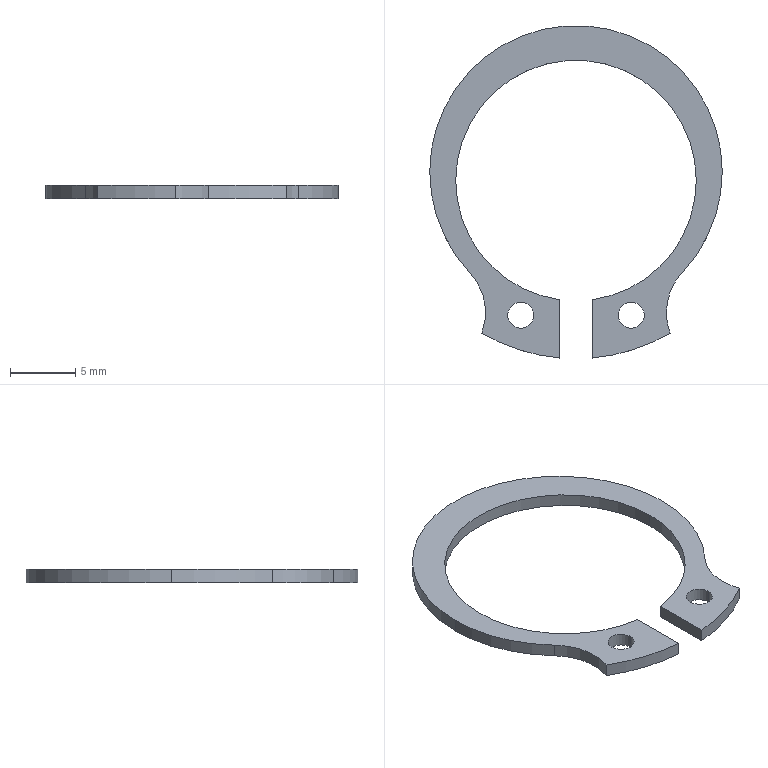Part | STEP file | 1 solid | 19 faces | box 22.5 x 25.566 x 1 mm | volume 158.597 mm3 | cylinder 15 | plane 4 | commonest cylinder face diameters 2 x4 9 x3 18.5 x3 22.5 x3 28.74 x2
STEP:
#1=CARTESIAN_POINT('',(3.25,-11.032,0.5));
#2=VERTEX_POINT('',#1);
#3=CARTESIAN_POINT('',(5.25,-11.032,0.5));
#4=VERTEX_POINT('',#3);
#5=CARTESIAN_POINT('',(4.25,-11.032,0.5));
#6=DIRECTION('',(0.,0.,1.));
#7=DIRECTION('',(-1.,0.,0.));
#8=AXIS2_PLACEMENT_3D('',#5,#6,#7);
#9=CIRCLE('',#8,1.);
#10=EDGE_CURVE('',#2,#4,#9,.T.);
#11=ORIENTED_EDGE('',*,*,#10,.T.);
#12=CARTESIAN_POINT('',(5.25,-11.032,-0.5));
#13=VERTEX_POINT('',#12);
#14=CARTESIAN_POINT('',(5.25,-11.032,0.5));
#15=DIRECTION('',(0.,0.,-1.));
#16=VECTOR('',#15,1000.);
#17=LINE('',#14,#16);
#18=EDGE_CURVE('',#4,#13,#17,.T.);
#19=ORIENTED_EDGE('',*,*,#18,.T.);
#20=CARTESIAN_POINT('',(3.25,-11.032,-0.5));
#21=VERTEX_POINT('',#20);
#22=CARTESIAN_POINT('',(4.25,-11.032,-0.5));
#23=DIRECTION('',(0.,0.,1.));
#24=DIRECTION('',(-1.,0.,0.));
#25=AXIS2_PLACEMENT_3D('',#22,#23,#24);
#26=CIRCLE('',#25,1.);
#27=EDGE_CURVE('',#21,#13,#26,.T.);
#28=ORIENTED_EDGE('',*,*,#27,.F.);
#29=CARTESIAN_POINT('',(3.25,-11.032,0.5));
#30=DIRECTION('',(0.,0.,-1.));
#31=VECTOR('',#30,1000.);
#32=LINE('',#29,#31);
#33=EDGE_CURVE('',#2,#21,#32,.T.);
#34=ORIENTED_EDGE('',*,*,#33,.F.);
#35=EDGE_LOOP('',(#11,#19,#28,#34));
#36=FACE_OUTER_BOUND('',#35,.T.);
#37=CARTESIAN_POINT('',(4.25,-11.032,0.5));
#38=DIRECTION('',(0.,0.,-1.));
#39=DIRECTION('',(-1.,0.,0.));
#40=AXIS2_PLACEMENT_3D('',#37,#38,#39);
#41=CYLINDRICAL_SURFACE('',#40,1.);
#42=ADVANCED_FACE('',(#36),#41,.F.);
#43=CARTESIAN_POINT('',(-5.25,-11.032,0.5));
#44=VERTEX_POINT('',#43);
#45=CARTESIAN_POINT('',(-3.25,-11.032,0.5));
#46=VERTEX_POINT('',#45);
#47=CARTESIAN_POINT('',(-4.25,-11.032,0.5));
#48=DIRECTION('',(0.,0.,1.));
#49=DIRECTION('',(1.,0.,0.));
#50=AXIS2_PLACEMENT_3D('',#47,#48,#49);
#51=CIRCLE('',#50,1.);
#52=EDGE_CURVE('',#44,#46,#51,.T.);
#53=ORIENTED_EDGE('',*,*,#52,.T.);
#54=CARTESIAN_POINT('',(-3.25,-11.032,-0.5));
#55=VERTEX_POINT('',#54);
#56=CARTESIAN_POINT('',(-3.25,-11.032,0.5));
#57=DIRECTION('',(0.,0.,-1.));
#58=VECTOR('',#57,1000.);
#59=LINE('',#56,#58);
#60=EDGE_CURVE('',#46,#55,#59,.T.);
#61=ORIENTED_EDGE('',*,*,#60,.T.);
#62=CARTESIAN_POINT('',(-5.25,-11.032,-0.5));
#63=VERTEX_POINT('',#62);
#64=CARTESIAN_POINT('',(-4.25,-11.032,-0.5));
#65=DIRECTION('',(0.,0.,1.));
#66=DIRECTION('',(1.,0.,0.));
#67=AXIS2_PLACEMENT_3D('',#64,#65,#66);
#68=CIRCLE('',#67,1.);
#69=EDGE_CURVE('',#63,#55,#68,.T.);
#70=ORIENTED_EDGE('',*,*,#69,.F.);
#71=CARTESIAN_POINT('',(-5.25,-11.032,0.5));
#72=DIRECTION('',(0.,0.,-1.));
#73=VECTOR('',#72,1000.);
#74=LINE('',#71,#73);
#75=EDGE_CURVE('',#44,#63,#74,.T.);
#76=ORIENTED_EDGE('',*,*,#75,.F.);
#77=EDGE_LOOP('',(#53,#61,#70,#76));
#78=FACE_OUTER_BOUND('',#77,.T.);
#79=CARTESIAN_POINT('',(-4.25,-11.032,0.5));
#80=DIRECTION('',(0.,0.,-1.));
#81=DIRECTION('',(-1.,0.,0.));
#82=AXIS2_PLACEMENT_3D('',#79,#80,#81);
#83=CYLINDRICAL_SURFACE('',#82,1.);
#84=ADVANCED_FACE('',(#78),#83,.F.);
#85=CARTESIAN_POINT('',(11.25,0.,0.5));
#86=VERTEX_POINT('',#85);
#87=CARTESIAN_POINT('',(-11.25,0.,0.5));
#88=VERTEX_POINT('',#87);
#89=CARTESIAN_POINT('',(0.,0.,0.5));
#90=DIRECTION('',(0.,0.,1.));
#91=DIRECTION('',(1.,0.,0.));
#92=AXIS2_PLACEMENT_3D('',#89,#90,#91);
#93=CIRCLE('',#92,11.25);
#94=EDGE_CURVE('',#86,#88,#93,.T.);
#95=ORIENTED_EDGE('',*,*,#94,.F.);
#96=CARTESIAN_POINT('',(11.25,0.,-0.5));
#97=VERTEX_POINT('',#96);
#98=CARTESIAN_POINT('',(11.25,0.,0.5));
#99=DIRECTION('',(0.,0.,-1.));
#100=VECTOR('',#99,1000.);
#101=LINE('',#98,#100);
#102=EDGE_CURVE('',#86,#97,#101,.T.);
#103=ORIENTED_EDGE('',*,*,#102,.T.);
#104=CARTESIAN_POINT('',(-11.25,0.,-0.5));
#105=VERTEX_POINT('',#104);
#106=CARTESIAN_POINT('',(0.,0.,-0.5));
#107=DIRECTION('',(0.,0.,1.));
#108=DIRECTION('',(1.,0.,0.));
#109=AXIS2_PLACEMENT_3D('',#106,#107,#108);
#110=CIRCLE('',#109,11.25);
#111=EDGE_CURVE('',#97,#105,#110,.T.);
#112=ORIENTED_EDGE('',*,*,#111,.T.);
#113=CARTESIAN_POINT('',(-11.25,0.,0.5));
#114=DIRECTION('',(0.,0.,-1.));
#115=VECTOR('',#114,1000.);
#116=LINE('',#113,#115);
#117=EDGE_CURVE('',#88,#105,#116,.T.);
#118=ORIENTED_EDGE('',*,*,#117,.F.);
#119=EDGE_LOOP('',(#95,#103,#112,#118));
#120=FACE_OUTER_BOUND('',#119,.T.);
#121=CARTESIAN_POINT('',(0.,0.,0.5));
#122=DIRECTION('',(0.,0.,-1.));
#123=DIRECTION('',(-1.,0.,0.));
#124=AXIS2_PLACEMENT_3D('',#121,#122,#123);
#125=CYLINDRICAL_SURFACE('',#124,11.25);
#126=ADVANCED_FACE('',(#120),#125,.T.);
#127=CARTESIAN_POINT('',(-8.183,-7.72,0.5));
#128=VERTEX_POINT('',#127);
#129=CARTESIAN_POINT('',(0.,0.,0.5));
#130=DIRECTION('',(0.,0.,1.));
#131=DIRECTION('',(1.,0.,0.));
#132=AXIS2_PLACEMENT_3D('',#129,#130,#131);
#133=CIRCLE('',#132,11.25);
#134=EDGE_CURVE('',#88,#128,#133,.T.);
#135=ORIENTED_EDGE('',*,*,#134,.F.);
#136=ORIENTED_EDGE('',*,*,#117,.T.);
#137=CARTESIAN_POINT('',(-8.183,-7.72,-0.5));
#138=VERTEX_POINT('',#137);
#139=CARTESIAN_POINT('',(0.,0.,-0.5));
#140=DIRECTION('',(0.,0.,1.));
#141=DIRECTION('',(1.,0.,0.));
#142=AXIS2_PLACEMENT_3D('',#139,#140,#141);
#143=CIRCLE('',#142,11.25);
#144=EDGE_CURVE('',#105,#138,#143,.T.);
#145=ORIENTED_EDGE('',*,*,#144,.T.);
#146=CARTESIAN_POINT('',(-8.183,-7.72,0.5));
#147=DIRECTION('',(0.,0.,-1.));
#148=VECTOR('',#147,1000.);
#149=LINE('',#146,#148);
#150=EDGE_CURVE('',#128,#138,#149,.T.);
#151=ORIENTED_EDGE('',*,*,#150,.F.);
#152=EDGE_LOOP('',(#135,#136,#145,#151));
#153=FACE_OUTER_BOUND('',#152,.T.);
#154=CARTESIAN_POINT('',(0.,0.,0.5));
#155=DIRECTION('',(0.,0.,-1.));
#156=DIRECTION('',(-1.,0.,0.));
#157=AXIS2_PLACEMENT_3D('',#154,#155,#156);
#158=CYLINDRICAL_SURFACE('',#157,11.25);
#159=ADVANCED_FACE('',(#153),#158,.T.);
#160=CARTESIAN_POINT('',(6.956,-10.808,0.5));
#161=VERTEX_POINT('',#160);
#162=CARTESIAN_POINT('',(8.183,-7.72,0.5));
#163=VERTEX_POINT('',#162);
#164=CARTESIAN_POINT('',(11.456,-10.808,0.5));
#165=DIRECTION('',(0.,0.,-1.));
#166=DIRECTION('',(-1.,0.,0.));
#167=AXIS2_PLACEMENT_3D('',#164,#165,#166);
#168=CIRCLE('',#167,4.5);
#169=EDGE_CURVE('',#161,#163,#168,.T.);
#170=ORIENTED_EDGE('',*,*,#169,.F.);
#171=CARTESIAN_POINT('',(6.956,-10.808,-0.5));
#172=VERTEX_POINT('',#171);
#173=CARTESIAN_POINT('',(6.956,-10.808,0.5));
#174=DIRECTION('',(0.,0.,-1.));
#175=VECTOR('',#174,1000.);
#176=LINE('',#173,#175);
#177=EDGE_CURVE('',#161,#172,#176,.T.);
#178=ORIENTED_EDGE('',*,*,#177,.T.);
#179=CARTESIAN_POINT('',(8.183,-7.72,-0.5));
#180=VERTEX_POINT('',#179);
#181=CARTESIAN_POINT('',(11.456,-10.808,-0.5));
#182=DIRECTION('',(0.,0.,-1.));
#183=DIRECTION('',(-1.,0.,0.));
#184=AXIS2_PLACEMENT_3D('',#181,#182,#183);
#185=CIRCLE('',#184,4.5);
#186=EDGE_CURVE('',#172,#180,#185,.T.);
#187=ORIENTED_EDGE('',*,*,#186,.T.);
#188=CARTESIAN_POINT('',(8.183,-7.72,0.5));
#189=DIRECTION('',(0.,0.,-1.));
#190=VECTOR('',#189,1000.);
#191=LINE('',#188,#190);
#192=EDGE_CURVE('',#163,#180,#191,.T.);
#193=ORIENTED_EDGE('',*,*,#192,.F.);
#194=EDGE_LOOP('',(#170,#178,#187,#193));
#195=FACE_OUTER_BOUND('',#194,.T.);
#196=CARTESIAN_POINT('',(11.456,-10.808,0.5));
#197=DIRECTION('',(0.,0.,-1.));
#198=DIRECTION('',(-1.,0.,0.));
#199=AXIS2_PLACEMENT_3D('',#196,#197,#198);
#200=CYLINDRICAL_SURFACE('',#199,4.5);
#201=ADVANCED_FACE('',(#195),#200,.F.);
#202=CARTESIAN_POINT('',(9.25,-0.67,0.5));
#203=VERTEX_POINT('',#202);
#204=CARTESIAN_POINT('',(1.25,-9.835,0.5));
#205=VERTEX_POINT('',#204);
#206=CARTESIAN_POINT('',(0.,-0.67,0.5));
#207=DIRECTION('',(0.,0.,-1.));
#208=DIRECTION('',(1.,0.,0.));
#209=AXIS2_PLACEMENT_3D('',#206,#207,#208);
#210=CIRCLE('',#209,9.25);
#211=EDGE_CURVE('',#203,#205,#210,.T.);
#212=ORIENTED_EDGE('',*,*,#211,.F.);
#213=CARTESIAN_POINT('',(9.25,-0.67,-0.5));
#214=VERTEX_POINT('',#213);
#215=CARTESIAN_POINT('',(9.25,-0.67,0.5));
#216=DIRECTION('',(0.,0.,-1.));
#217=VECTOR('',#216,1000.);
#218=LINE('',#215,#217);
#219=EDGE_CURVE('',#203,#214,#218,.T.);
#220=ORIENTED_EDGE('',*,*,#219,.T.);
#221=CARTESIAN_POINT('',(1.25,-9.835,-0.5));
#222=VERTEX_POINT('',#221);
#223=CARTESIAN_POINT('',(0.,-0.67,-0.5));
#224=DIRECTION('',(0.,0.,-1.));
#225=DIRECTION('',(1.,0.,0.));
#226=AXIS2_PLACEMENT_3D('',#223,#224,#225);
#227=CIRCLE('',#226,9.25);
#228=EDGE_CURVE('',#214,#222,#227,.T.);
#229=ORIENTED_EDGE('',*,*,#228,.T.);
#230=CARTESIAN_POINT('',(1.25,-9.835,0.5));
#231=DIRECTION('',(0.,0.,-1.));
#232=VECTOR('',#231,1000.);
#233=LINE('',#230,#232);
#234=EDGE_CURVE('',#205,#222,#233,.T.);
#235=ORIENTED_EDGE('',*,*,#234,.F.);
#236=EDGE_LOOP('',(#212,#220,#229,#235));
#237=FACE_OUTER_BOUND('',#236,.T.);
#238=CARTESIAN_POINT('',(0.,-0.67,0.5));
#239=DIRECTION('',(0.,0.,-1.));
#240=DIRECTION('',(-1.,0.,0.));
#241=AXIS2_PLACEMENT_3D('',#238,#239,#240);
#242=CYLINDRICAL_SURFACE('',#241,9.25);
#243=ADVANCED_FACE('',(#237),#242,.F.);
#244=ORIENTED_EDGE('',*,*,#219,.F.);
#245=CARTESIAN_POINT('',(-9.25,-0.67,0.5));
#246=VERTEX_POINT('',#245);
#247=CARTESIAN_POINT('',(0.,-0.67,0.5));
#248=DIRECTION('',(0.,0.,-1.));
#249=DIRECTION('',(1.,0.,0.));
#250=AXIS2_PLACEMENT_3D('',#247,#248,#249);
#251=CIRCLE('',#250,9.25);
#252=EDGE_CURVE('',#246,#203,#251,.T.);
#253=ORIENTED_EDGE('',*,*,#252,.F.);
#254=CARTESIAN_POINT('',(-9.25,-0.67,-0.5));
#255=VERTEX_POINT('',#254);
#256=CARTESIAN_POINT('',(-9.25,-0.67,0.5));
#257=DIRECTION('',(0.,0.,-1.));
#258=VECTOR('',#257,1000.);
#259=LINE('',#256,#258);
#260=EDGE_CURVE('',#246,#255,#259,.T.);
#261=ORIENTED_EDGE('',*,*,#260,.T.);
#262=CARTESIAN_POINT('',(0.,-0.67,-0.5));
#263=DIRECTION('',(0.,0.,-1.));
#264=DIRECTION('',(1.,0.,0.));
#265=AXIS2_PLACEMENT_3D('',#262,#263,#264);
#266=CIRCLE('',#265,9.25);
#267=EDGE_CURVE('',#255,#214,#266,.T.);
#268=ORIENTED_EDGE('',*,*,#267,.T.);
#269=EDGE_LOOP('',(#244,#253,#261,#268));
#270=FACE_OUTER_BOUND('',#269,.T.);
#271=CARTESIAN_POINT('',(0.,-0.67,0.5));
#272=DIRECTION('',(0.,0.,-1.));
#273=DIRECTION('',(-1.,0.,0.));
#274=AXIS2_PLACEMENT_3D('',#271,#272,#273);
#275=CYLINDRICAL_SURFACE('',#274,9.25);
#276=ADVANCED_FACE('',(#270),#275,.F.);
#277=ORIENTED_EDGE('',*,*,#52,.F.);
#278=CARTESIAN_POINT('',(-4.25,-11.032,0.5));
#279=DIRECTION('',(0.,0.,1.));
#280=DIRECTION('',(1.,0.,0.));
#281=AXIS2_PLACEMENT_3D('',#278,#279,#280);
#282=CIRCLE('',#281,1.);
#283=EDGE_CURVE('',#46,#44,#282,.T.);
#284=ORIENTED_EDGE('',*,*,#283,.F.);
#285=EDGE_LOOP('',(#277,#284));
#286=FACE_BOUND('',#285,.T.);
#287=CARTESIAN_POINT('',(-1.25,-9.835,0.5));
#288=VERTEX_POINT('',#287);
#289=CARTESIAN_POINT('',(0.,-0.67,0.5));
#290=DIRECTION('',(0.,0.,-1.));
#291=DIRECTION('',(1.,0.,0.));
#292=AXIS2_PLACEMENT_3D('',#289,#290,#291);
#293=CIRCLE('',#292,9.25);
#294=EDGE_CURVE('',#288,#246,#293,.T.);
#295=ORIENTED_EDGE('',*,*,#294,.T.);
#296=ORIENTED_EDGE('',*,*,#252,.T.);
#297=ORIENTED_EDGE('',*,*,#211,.T.);
#298=CARTESIAN_POINT('',(1.25,-14.316,0.5));
#299=VERTEX_POINT('',#298);
#300=CARTESIAN_POINT('',(1.25,-9.835,0.5));
#301=DIRECTION('',(0.,-1.,0.));
#302=VECTOR('',#301,1000.);
#303=LINE('',#300,#302);
#304=EDGE_CURVE('',#205,#299,#303,.T.);
#305=ORIENTED_EDGE('',*,*,#304,.T.);
#306=CARTESIAN_POINT('',(7.25,-12.407,0.5));
#307=VERTEX_POINT('',#306);
#308=CARTESIAN_POINT('',(0.,0.,0.5));
#309=DIRECTION('',(0.,0.,1.));
#310=DIRECTION('',(1.,0.,0.));
#311=AXIS2_PLACEMENT_3D('',#308,#309,#310);
#312=CIRCLE('',#311,14.37);
#313=EDGE_CURVE('',#299,#307,#312,.T.);
#314=ORIENTED_EDGE('',*,*,#313,.T.);
#315=CARTESIAN_POINT('',(11.456,-10.808,0.5));
#316=DIRECTION('',(0.,0.,-1.));
#317=DIRECTION('',(-1.,0.,0.));
#318=AXIS2_PLACEMENT_3D('',#315,#316,#317);
#319=CIRCLE('',#318,4.5);
#320=EDGE_CURVE('',#307,#161,#319,.T.);
#321=ORIENTED_EDGE('',*,*,#320,.T.);
#322=ORIENTED_EDGE('',*,*,#169,.T.);
#323=CARTESIAN_POINT('',(0.,0.,0.5));
#324=DIRECTION('',(0.,0.,1.));
#325=DIRECTION('',(1.,0.,0.));
#326=AXIS2_PLACEMENT_3D('',#323,#324,#325);
#327=CIRCLE('',#326,11.25);
#328=EDGE_CURVE('',#163,#86,#327,.T.);
#329=ORIENTED_EDGE('',*,*,#328,.T.);
#330=ORIENTED_EDGE('',*,*,#94,.T.);
#331=ORIENTED_EDGE('',*,*,#134,.T.);
#332=CARTESIAN_POINT('',(-7.25,-12.407,0.5));
#333=VERTEX_POINT('',#332);
#334=CARTESIAN_POINT('',(-11.456,-10.808,0.5));
#335=DIRECTION('',(0.,0.,-1.));
#336=DIRECTION('',(1.,0.,0.));
#337=AXIS2_PLACEMENT_3D('',#334,#335,#336);
#338=CIRCLE('',#337,4.5);
#339=EDGE_CURVE('',#128,#333,#338,.T.);
#340=ORIENTED_EDGE('',*,*,#339,.T.);
#341=CARTESIAN_POINT('',(-1.25,-14.316,0.5));
#342=VERTEX_POINT('',#341);
#343=CARTESIAN_POINT('',(0.,0.,0.5));
#344=DIRECTION('',(0.,0.,1.));
#345=DIRECTION('',(-1.,0.,0.));
#346=AXIS2_PLACEMENT_3D('',#343,#344,#345);
#347=CIRCLE('',#346,14.37);
#348=EDGE_CURVE('',#333,#342,#347,.T.);
#349=ORIENTED_EDGE('',*,*,#348,.T.);
#350=CARTESIAN_POINT('',(-1.25,-9.835,0.5));
#351=DIRECTION('',(0.,1.,0.));
#352=VECTOR('',#351,1000.);
#353=LINE('',#350,#352);
#354=EDGE_CURVE('',#342,#288,#353,.T.);
#355=ORIENTED_EDGE('',*,*,#354,.T.);
#356=EDGE_LOOP('',(#295,#296,#297,#305,#314,#321,#322,#329,#330,#331,#340,#349,#355));
#357=FACE_OUTER_BOUND('',#356,.T.);
#358=ORIENTED_EDGE('',*,*,#10,.F.);
#359=CARTESIAN_POINT('',(4.25,-11.032,0.5));
#360=DIRECTION('',(0.,0.,1.));
#361=DIRECTION('',(-1.,0.,0.));
#362=AXIS2_PLACEMENT_3D('',#359,#360,#361);
#363=CIRCLE('',#362,1.);
#364=EDGE_CURVE('',#4,#2,#363,.T.);
#365=ORIENTED_EDGE('',*,*,#364,.F.);
#366=EDGE_LOOP('',(#358,#365));
#367=FACE_BOUND('',#366,.T.);
#368=CARTESIAN_POINT('',(0.,-0.67,0.5));
#369=DIRECTION('',(0.,0.,1.));
#370=DIRECTION('',(1.,0.,0.));
#371=AXIS2_PLACEMENT_3D('',#368,#369,#370);
#372=PLANE('',#371);
#373=ADVANCED_FACE('',(#286,#357,#367),#372,.T.);
#374=ORIENTED_EDGE('',*,*,#260,.F.);
#375=ORIENTED_EDGE('',*,*,#294,.F.);
#376=CARTESIAN_POINT('',(-1.25,-9.835,-0.5));
#377=VERTEX_POINT('',#376);
#378=CARTESIAN_POINT('',(-1.25,-9.835,0.5));
#379=DIRECTION('',(0.,0.,-1.));
#380=VECTOR('',#379,1000.);
#381=LINE('',#378,#380);
#382=EDGE_CURVE('',#288,#377,#381,.T.);
#383=ORIENTED_EDGE('',*,*,#382,.T.);
#384=CARTESIAN_POINT('',(0.,-0.67,-0.5));
#385=DIRECTION('',(0.,0.,-1.));
#386=DIRECTION('',(1.,0.,0.));
#387=AXIS2_PLACEMENT_3D('',#384,#385,#386);
#388=CIRCLE('',#387,9.25);
#389=EDGE_CURVE('',#377,#255,#388,.T.);
#390=ORIENTED_EDGE('',*,*,#389,.T.);
#391=EDGE_LOOP('',(#374,#375,#383,#390));
#392=FACE_OUTER_BOUND('',#391,.T.);
#393=CARTESIAN_POINT('',(0.,-0.67,0.5));
#394=DIRECTION('',(0.,0.,-1.));
#395=DIRECTION('',(-1.,0.,0.));
#396=AXIS2_PLACEMENT_3D('',#393,#394,#395);
#397=CYLINDRICAL_SURFACE('',#396,9.25);
#398=ADVANCED_FACE('',(#392),#397,.F.);
#399=ORIENTED_EDGE('',*,*,#234,.T.);
#400=CARTESIAN_POINT('',(1.25,-14.316,-0.5));
#401=VERTEX_POINT('',#400);
#402=CARTESIAN_POINT('',(1.25,-9.835,-0.5));
#403=DIRECTION('',(0.,-1.,0.));
#404=VECTOR('',#403,1000.);
#405=LINE('',#402,#404);
#406=EDGE_CURVE('',#222,#401,#405,.T.);
#407=ORIENTED_EDGE('',*,*,#406,.T.);
#408=CARTESIAN_POINT('',(1.25,-14.316,0.5));
#409=DIRECTION('',(0.,0.,-1.));
#410=VECTOR('',#409,1000.);
#411=LINE('',#408,#410);
#412=EDGE_CURVE('',#299,#401,#411,.T.);
#413=ORIENTED_EDGE('',*,*,#412,.F.);
#414=ORIENTED_EDGE('',*,*,#304,.F.);
#415=EDGE_LOOP('',(#399,#407,#413,#414));
#416=FACE_OUTER_BOUND('',#415,.T.);
#417=CARTESIAN_POINT('',(1.25,-9.835,0.5));
#418=DIRECTION('',(1.,0.,0.));
#419=DIRECTION('',(0.,1.,0.));
#420=AXIS2_PLACEMENT_3D('',#417,#418,#419);
#421=PLANE('',#420);
#422=ADVANCED_FACE('',(#416),#421,.F.);
#423=ORIENTED_EDGE('',*,*,#412,.T.);
#424=CARTESIAN_POINT('',(7.25,-12.407,-0.5));
#425=VERTEX_POINT('',#424);
#426=CARTESIAN_POINT('',(0.,0.,-0.5));
#427=DIRECTION('',(0.,0.,1.));
#428=DIRECTION('',(1.,0.,0.));
#429=AXIS2_PLACEMENT_3D('',#426,#427,#428);
#430=CIRCLE('',#429,14.37);
#431=EDGE_CURVE('',#401,#425,#430,.T.);
#432=ORIENTED_EDGE('',*,*,#431,.T.);
#433=CARTESIAN_POINT('',(7.25,-12.407,0.5));
#434=DIRECTION('',(0.,0.,-1.));
#435=VECTOR('',#434,1000.);
#436=LINE('',#433,#435);
#437=EDGE_CURVE('',#307,#425,#436,.T.);
#438=ORIENTED_EDGE('',*,*,#437,.F.);
#439=ORIENTED_EDGE('',*,*,#313,.F.);
#440=EDGE_LOOP('',(#423,#432,#438,#439));
#441=FACE_OUTER_BOUND('',#440,.T.);
#442=CARTESIAN_POINT('',(0.,0.,0.5));
#443=DIRECTION('',(0.,0.,-1.));
#444=DIRECTION('',(-1.,0.,0.));
#445=AXIS2_PLACEMENT_3D('',#442,#443,#444);
#446=CYLINDRICAL_SURFACE('',#445,14.37);
#447=ADVANCED_FACE('',(#441),#446,.T.);
#448=ORIENTED_EDGE('',*,*,#177,.F.);
#449=ORIENTED_EDGE('',*,*,#320,.F.);
#450=ORIENTED_EDGE('',*,*,#437,.T.);
#451=CARTESIAN_POINT('',(11.456,-10.808,-0.5));
#452=DIRECTION('',(0.,0.,-1.));
#453=DIRECTION('',(-1.,0.,0.));
#454=AXIS2_PLACEMENT_3D('',#451,#452,#453);
#455=CIRCLE('',#454,4.5);
#456=EDGE_CURVE('',#425,#172,#455,.T.);
#457=ORIENTED_EDGE('',*,*,#456,.T.);
#458=EDGE_LOOP('',(#448,#449,#450,#457));
#459=FACE_OUTER_BOUND('',#458,.T.);
#460=CARTESIAN_POINT('',(11.456,-10.808,0.5));
#461=DIRECTION('',(0.,0.,-1.));
#462=DIRECTION('',(-1.,0.,0.));
#463=AXIS2_PLACEMENT_3D('',#460,#461,#462);
#464=CYLINDRICAL_SURFACE('',#463,4.5);
#465=ADVANCED_FACE('',(#459),#464,.F.);
#466=ORIENTED_EDGE('',*,*,#102,.F.);
#467=ORIENTED_EDGE('',*,*,#328,.F.);
#468=ORIENTED_EDGE('',*,*,#192,.T.);
#469=CARTESIAN_POINT('',(0.,0.,-0.5));
#470=DIRECTION('',(0.,0.,1.));
#471=DIRECTION('',(1.,0.,0.));
#472=AXIS2_PLACEMENT_3D('',#469,#470,#471);
#473=CIRCLE('',#472,11.25);
#474=EDGE_CURVE('',#180,#97,#473,.T.);
#475=ORIENTED_EDGE('',*,*,#474,.T.);
#476=EDGE_LOOP('',(#466,#467,#468,#475));
#477=FACE_OUTER_BOUND('',#476,.T.);
#478=CARTESIAN_POINT('',(0.,0.,0.5));
#479=DIRECTION('',(0.,0.,-1.));
#480=DIRECTION('',(-1.,0.,0.));
#481=AXIS2_PLACEMENT_3D('',#478,#479,#480);
#482=CYLINDRICAL_SURFACE('',#481,11.25);
#483=ADVANCED_FACE('',(#477),#482,.T.);
#484=ORIENTED_EDGE('',*,*,#150,.T.);
#485=CARTESIAN_POINT('',(-7.25,-12.407,-0.5));
#486=VERTEX_POINT('',#485);
#487=CARTESIAN_POINT('',(-11.456,-10.808,-0.5));
#488=DIRECTION('',(0.,0.,-1.));
#489=DIRECTION('',(1.,0.,0.));
#490=AXIS2_PLACEMENT_3D('',#487,#488,#489);
#491=CIRCLE('',#490,4.5);
#492=EDGE_CURVE('',#138,#486,#491,.T.);
#493=ORIENTED_EDGE('',*,*,#492,.T.);
#494=CARTESIAN_POINT('',(-7.25,-12.407,0.5));
#495=DIRECTION('',(0.,0.,-1.));
#496=VECTOR('',#495,1000.);
#497=LINE('',#494,#496);
#498=EDGE_CURVE('',#333,#486,#497,.T.);
#499=ORIENTED_EDGE('',*,*,#498,.F.);
#500=ORIENTED_EDGE('',*,*,#339,.F.);
#501=EDGE_LOOP('',(#484,#493,#499,#500));
#502=FACE_OUTER_BOUND('',#501,.T.);
#503=CARTESIAN_POINT('',(-11.456,-10.808,0.5));
#504=DIRECTION('',(0.,0.,-1.));
#505=DIRECTION('',(-1.,0.,0.));
#506=AXIS2_PLACEMENT_3D('',#503,#504,#505);
#507=CYLINDRICAL_SURFACE('',#506,4.5);
#508=ADVANCED_FACE('',(#502),#507,.F.);
#509=ORIENTED_EDGE('',*,*,#498,.T.);
#510=CARTESIAN_POINT('',(-1.25,-14.316,-0.5));
#511=VERTEX_POINT('',#510);
#512=CARTESIAN_POINT('',(0.,0.,-0.5));
#513=DIRECTION('',(0.,0.,1.));
#514=DIRECTION('',(-1.,0.,0.));
#515=AXIS2_PLACEMENT_3D('',#512,#513,#514);
#516=CIRCLE('',#515,14.37);
#517=EDGE_CURVE('',#486,#511,#516,.T.);
#518=ORIENTED_EDGE('',*,*,#517,.T.);
#519=CARTESIAN_POINT('',(-1.25,-14.316,0.5));
#520=DIRECTION('',(0.,0.,-1.));
#521=VECTOR('',#520,1000.);
#522=LINE('',#519,#521);
#523=EDGE_CURVE('',#342,#511,#522,.T.);
#524=ORIENTED_EDGE('',*,*,#523,.F.);
#525=ORIENTED_EDGE('',*,*,#348,.F.);
#526=EDGE_LOOP('',(#509,#518,#524,#525));
#527=FACE_OUTER_BOUND('',#526,.T.);
#528=CARTESIAN_POINT('',(0.,0.,0.5));
#529=DIRECTION('',(0.,0.,-1.));
#530=DIRECTION('',(-1.,0.,0.));
#531=AXIS2_PLACEMENT_3D('',#528,#529,#530);
#532=CYLINDRICAL_SURFACE('',#531,14.37);
#533=ADVANCED_FACE('',(#527),#532,.T.);
#534=ORIENTED_EDGE('',*,*,#523,.T.);
#535=CARTESIAN_POINT('',(-1.25,-9.835,-0.5));
#536=DIRECTION('',(0.,1.,0.));
#537=VECTOR('',#536,1000.);
#538=LINE('',#535,#537);
#539=EDGE_CURVE('',#511,#377,#538,.T.);
#540=ORIENTED_EDGE('',*,*,#539,.T.);
#541=ORIENTED_EDGE('',*,*,#382,.F.);
#542=ORIENTED_EDGE('',*,*,#354,.F.);
#543=EDGE_LOOP('',(#534,#540,#541,#542));
#544=FACE_OUTER_BOUND('',#543,.T.);
#545=CARTESIAN_POINT('',(-1.25,-9.835,0.5));
#546=DIRECTION('',(-1.,0.,0.));
#547=DIRECTION('',(0.,-1.,0.));
#548=AXIS2_PLACEMENT_3D('',#545,#546,#547);
#549=PLANE('',#548);
#550=ADVANCED_FACE('',(#544),#549,.F.);
#551=ORIENTED_EDGE('',*,*,#60,.F.);
#552=ORIENTED_EDGE('',*,*,#283,.T.);
#553=ORIENTED_EDGE('',*,*,#75,.T.);
#554=CARTESIAN_POINT('',(-4.25,-11.032,-0.5));
#555=DIRECTION('',(0.,0.,1.));
#556=DIRECTION('',(1.,0.,0.));
#557=AXIS2_PLACEMENT_3D('',#554,#555,#556);
#558=CIRCLE('',#557,1.);
#559=EDGE_CURVE('',#55,#63,#558,.T.);
#560=ORIENTED_EDGE('',*,*,#559,.F.);
#561=EDGE_LOOP('',(#551,#552,#553,#560));
#562=FACE_OUTER_BOUND('',#561,.T.);
#563=CARTESIAN_POINT('',(-4.25,-11.032,0.5));
#564=DIRECTION('',(0.,0.,-1.));
#565=DIRECTION('',(-1.,0.,0.));
#566=AXIS2_PLACEMENT_3D('',#563,#564,#565);
#567=CYLINDRICAL_SURFACE('',#566,1.);
#568=ADVANCED_FACE('',(#562),#567,.F.);
#569=ORIENTED_EDGE('',*,*,#18,.F.);
#570=ORIENTED_EDGE('',*,*,#364,.T.);
#571=ORIENTED_EDGE('',*,*,#33,.T.);
#572=CARTESIAN_POINT('',(4.25,-11.032,-0.5));
#573=DIRECTION('',(0.,0.,1.));
#574=DIRECTION('',(-1.,0.,0.));
#575=AXIS2_PLACEMENT_3D('',#572,#573,#574);
#576=CIRCLE('',#575,1.);
#577=EDGE_CURVE('',#13,#21,#576,.T.);
#578=ORIENTED_EDGE('',*,*,#577,.F.);
#579=EDGE_LOOP('',(#569,#570,#571,#578));
#580=FACE_OUTER_BOUND('',#579,.T.);
#581=CARTESIAN_POINT('',(4.25,-11.032,0.5));
#582=DIRECTION('',(0.,0.,-1.));
#583=DIRECTION('',(-1.,0.,0.));
#584=AXIS2_PLACEMENT_3D('',#581,#582,#583);
#585=CYLINDRICAL_SURFACE('',#584,1.);
#586=ADVANCED_FACE('',(#580),#585,.F.);
#587=ORIENTED_EDGE('',*,*,#27,.T.);
#588=ORIENTED_EDGE('',*,*,#577,.T.);
#589=EDGE_LOOP('',(#587,#588));
#590=FACE_BOUND('',#589,.T.);
#591=ORIENTED_EDGE('',*,*,#69,.T.);
#592=ORIENTED_EDGE('',*,*,#559,.T.);
#593=EDGE_LOOP('',(#591,#592));
#594=FACE_BOUND('',#593,.T.);
#595=ORIENTED_EDGE('',*,*,#389,.F.);
#596=ORIENTED_EDGE('',*,*,#539,.F.);
#597=ORIENTED_EDGE('',*,*,#517,.F.);
#598=ORIENTED_EDGE('',*,*,#492,.F.);
#599=ORIENTED_EDGE('',*,*,#144,.F.);
#600=ORIENTED_EDGE('',*,*,#111,.F.);
#601=ORIENTED_EDGE('',*,*,#474,.F.);
#602=ORIENTED_EDGE('',*,*,#186,.F.);
#603=ORIENTED_EDGE('',*,*,#456,.F.);
#604=ORIENTED_EDGE('',*,*,#431,.F.);
#605=ORIENTED_EDGE('',*,*,#406,.F.);
#606=ORIENTED_EDGE('',*,*,#228,.F.);
#607=ORIENTED_EDGE('',*,*,#267,.F.);
#608=EDGE_LOOP('',(#595,#596,#597,#598,#599,#600,#601,#602,#603,#604,#605,#606,#607));
#609=FACE_OUTER_BOUND('',#608,.T.);
#610=CARTESIAN_POINT('',(0.,-0.67,-0.5));
#611=DIRECTION('',(0.,0.,1.));
#612=DIRECTION('',(1.,0.,0.));
#613=AXIS2_PLACEMENT_3D('',#610,#611,#612);
#614=PLANE('',#613);
#615=ADVANCED_FACE('',(#590,#594,#609),#614,.F.);
#616=CLOSED_SHELL('',(#42,#84,#126,#159,#201,#243,#276,#373,#398,#422,#447,#465,#483,#508,#533,#550,#568,#586,#615));
#617=MANIFOLD_SOLID_BREP('',#616);
#618=CARTESIAN_POINT('',(0.,0.,0.));
#619=DIRECTION('',(0.,0.,1.));
#620=DIRECTION('',(1.,0.,0.));
#621=AXIS2_PLACEMENT_3D('',#618,#619,#620);
#622=(LENGTH_UNIT()NAMED_UNIT(*)SI_UNIT(.MILLI.,.METRE.));
#623=UNCERTAINTY_MEASURE_WITH_UNIT(LENGTH_MEASURE(0.00001),#622,'','');
#624=(NAMED_UNIT(*)PLANE_ANGLE_UNIT()SI_UNIT($,.RADIAN.));
#625=(NAMED_UNIT(*)SI_UNIT($,.STERADIAN.)SOLID_ANGLE_UNIT());
#626=(GEOMETRIC_REPRESENTATION_CONTEXT(3)GLOBAL_UNCERTAINTY_ASSIGNED_CONTEXT((#623))GLOBAL_UNIT_ASSIGNED_CONTEXT((#622,#624,#625))REPRESENTATION_CONTEXT('',''));
#627=ADVANCED_BREP_SHAPE_REPRESENTATION('',(#617,#621),#626);